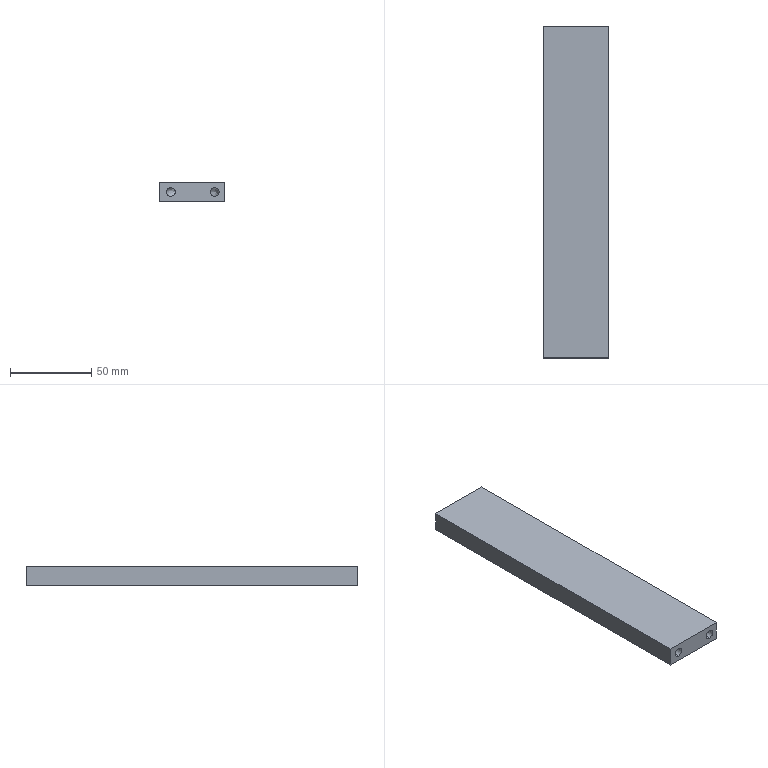Part | SolidWorks | features BaseBody 1 | 1 solid | 32 faces | box 40 x 204 x 12 mm | volume 79693 mm3 | spline 26 | plane 6